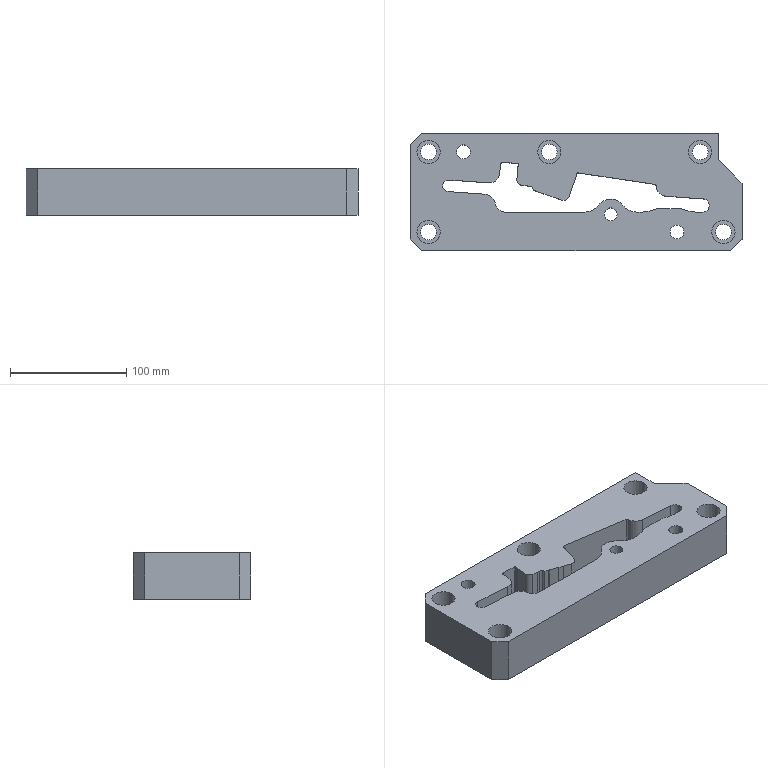Part | NX | features 23 2 | 1 solid | 79 faces | box 286 x 101 x 40 mm | volume 892651 mm3 | plane 41 | cylinder 38 | commonest cylinder face diameters 2 x6 20 x6 13.5 x5 40 x4 4 x2 10 x2